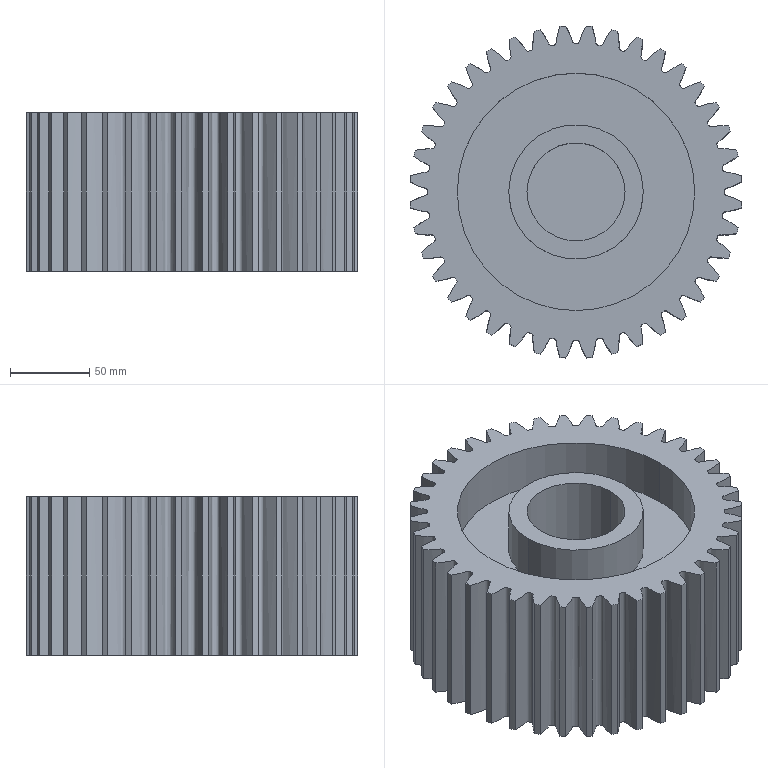Part | SolidWorks | 1 solid | 102 faces | box 209.617 x 209.617 x 100 mm | volume 2166914 mm3 | cylinder 52 | spline 40 | plane 10 | commonest cylinder face diameters 210 x40 85 x4 150 x4 40 x2 62 x2